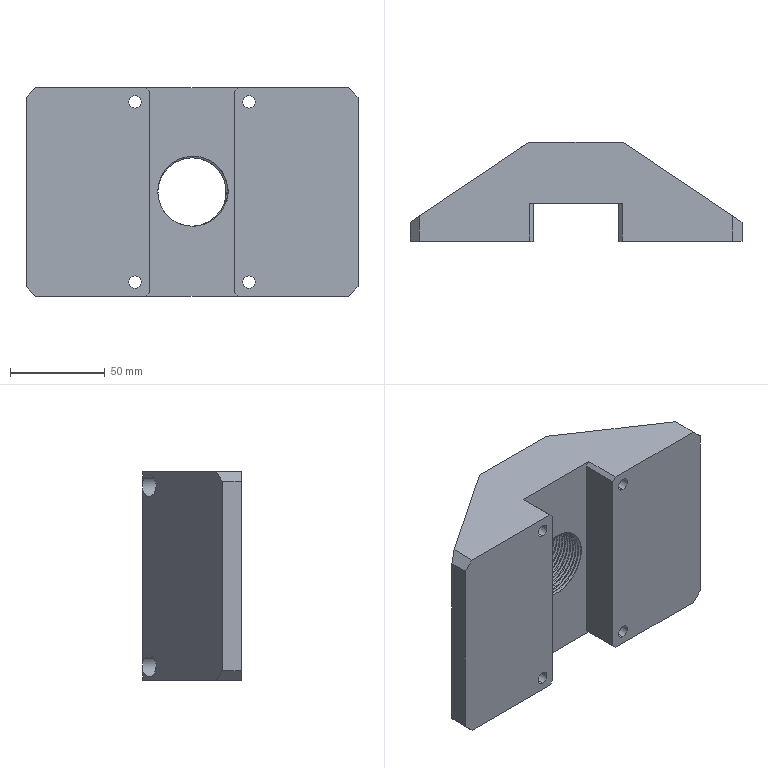Part | SolidWorks | features BaseBody 1 | 1 solid | 77 faces | box 175 x 52 x 110 mm | volume 567530 mm3 | cylinder 49 | plane 25 | spline 3 | commonest cylinder face diameters 36 x33 6.6 x8 11 x8